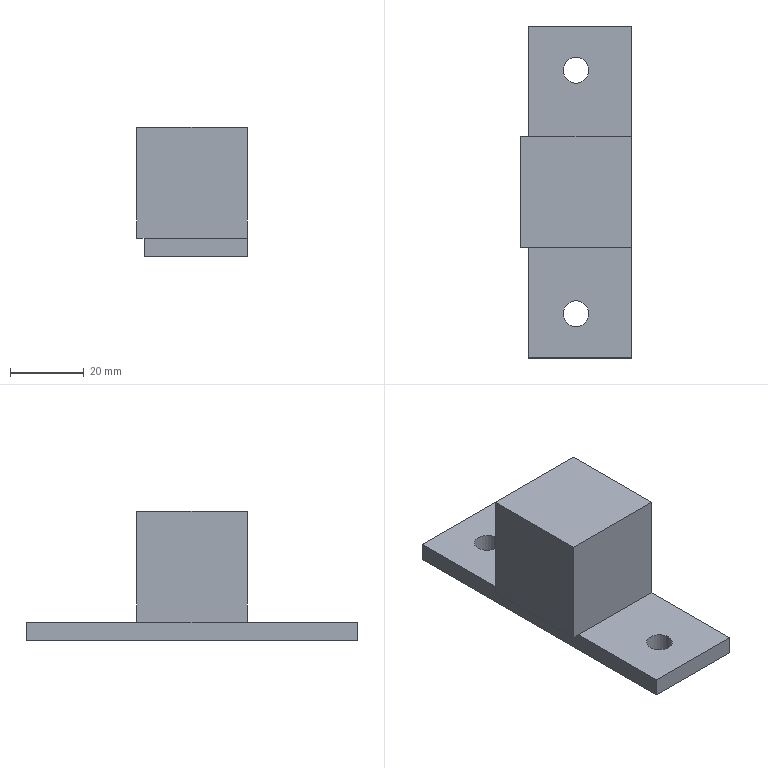Part | STEP file | diancitie | 1 solid | 14 faces | box 30 x 90 x 35 mm | volume 39215 mm3 | plane 12 | cylinder 2 | commonest cylinder face diameters 7 x2
STEP:
#1=CARTESIAN_POINT('',(0.,0.,0.));
#2=DIRECTION('',(0.,0.,1.));
#3=DIRECTION('',(1.,0.,0.));
#4=AXIS2_PLACEMENT_3D('',#1,#2,#3);
#5=CARTESIAN_POINT('',(-14.,-45.,0.));
#6=VERTEX_POINT('',#5);
#7=CARTESIAN_POINT('',(14.,-45.,0.));
#8=VERTEX_POINT('',#7);
#9=CARTESIAN_POINT('',(0.,-45.,0.));
#10=DIRECTION('',(1.,0.,0.));
#11=VECTOR('',#10,1.);
#12=LINE('',#9,#11);
#13=CARTESIAN_POINT('',(0.,0.,0.));
#14=DIRECTION('',(0.,0.,1.));
#15=DIRECTION('',(1.,0.,0.));
#16=AXIS2_PLACEMENT_3D('',#13,#14,#15);
#17=PLANE('',#16);
#18=CARTESIAN_POINT('',(0.,-45.));
#19=DIRECTION('',(1.,0.));
#20=VECTOR('',#19,1.);
#21=LINE('',#18,#20);
#22=(GEOMETRIC_REPRESENTATION_CONTEXT(2)PARAMETRIC_REPRESENTATION_CONTEXT()REPRESENTATION_CONTEXT('',''));
#23=DEFINITIONAL_REPRESENTATION('',(#21),#22);
#24=PCURVE('',#17,#23);
#25=CARTESIAN_POINT('',(-14.,-45.,5.));
#26=DIRECTION('',(0.,1.,0.));
#27=DIRECTION('',(0.,0.,1.));
#28=AXIS2_PLACEMENT_3D('',#25,#26,#27);
#29=PLANE('',#28);
#30=CARTESIAN_POINT('',(-5.,14.));
#31=DIRECTION('',(0.,1.));
#32=VECTOR('',#31,1.);
#33=LINE('',#30,#32);
#34=(GEOMETRIC_REPRESENTATION_CONTEXT(2)PARAMETRIC_REPRESENTATION_CONTEXT()REPRESENTATION_CONTEXT('',''));
#35=DEFINITIONAL_REPRESENTATION('',(#33),#34);
#36=PCURVE('',#29,#35);
#37=SURFACE_CURVE('',#12,(#24,#36),.PCURVE_S1.);
#38=EDGE_CURVE('',#6,#8,#37,.T.);
#39=ORIENTED_EDGE('',*,*,#38,.F.);
#40=CARTESIAN_POINT('',(-14.,45.,0.));
#41=VERTEX_POINT('',#40);
#42=CARTESIAN_POINT('',(-14.,0.,0.));
#43=DIRECTION('',(0.,-1.,0.));
#44=VECTOR('',#43,1.);
#45=LINE('',#42,#44);
#46=CARTESIAN_POINT('',(-14.,0.));
#47=DIRECTION('',(0.,-1.));
#48=VECTOR('',#47,1.);
#49=LINE('',#46,#48);
#50=(GEOMETRIC_REPRESENTATION_CONTEXT(2)PARAMETRIC_REPRESENTATION_CONTEXT()REPRESENTATION_CONTEXT('',''));
#51=DEFINITIONAL_REPRESENTATION('',(#49),#50);
#52=PCURVE('',#17,#51);
#53=CARTESIAN_POINT('',(-14.,45.,5.));
#54=DIRECTION('',(1.,0.,0.));
#55=DIRECTION('',(0.,1.,0.));
#56=AXIS2_PLACEMENT_3D('',#53,#54,#55);
#57=PLANE('',#56);
#58=CARTESIAN_POINT('',(-45.,-5.));
#59=DIRECTION('',(-1.,0.));
#60=VECTOR('',#59,1.);
#61=LINE('',#58,#60);
#62=(GEOMETRIC_REPRESENTATION_CONTEXT(2)PARAMETRIC_REPRESENTATION_CONTEXT()REPRESENTATION_CONTEXT('',''));
#63=DEFINITIONAL_REPRESENTATION('',(#61),#62);
#64=PCURVE('',#57,#63);
#65=SURFACE_CURVE('',#45,(#52,#64),.PCURVE_S1.);
#66=EDGE_CURVE('',#41,#6,#65,.T.);
#67=ORIENTED_EDGE('',*,*,#66,.F.);
#68=CARTESIAN_POINT('',(14.,45.,0.));
#69=VERTEX_POINT('',#68);
#70=CARTESIAN_POINT('',(0.,45.,0.));
#71=DIRECTION('',(-1.,0.,0.));
#72=VECTOR('',#71,1.);
#73=LINE('',#70,#72);
#74=CARTESIAN_POINT('',(0.,45.));
#75=DIRECTION('',(-1.,0.));
#76=VECTOR('',#75,1.);
#77=LINE('',#74,#76);
#78=(GEOMETRIC_REPRESENTATION_CONTEXT(2)PARAMETRIC_REPRESENTATION_CONTEXT()REPRESENTATION_CONTEXT('',''));
#79=DEFINITIONAL_REPRESENTATION('',(#77),#78);
#80=PCURVE('',#17,#79);
#81=CARTESIAN_POINT('',(-14.,45.,5.));
#82=DIRECTION('',(0.,-1.,0.));
#83=DIRECTION('',(0.,0.,-1.));
#84=AXIS2_PLACEMENT_3D('',#81,#82,#83);
#85=PLANE('',#84);
#86=CARTESIAN_POINT('',(5.,14.));
#87=DIRECTION('',(0.,-1.));
#88=VECTOR('',#87,1.);
#89=LINE('',#86,#88);
#90=(GEOMETRIC_REPRESENTATION_CONTEXT(2)PARAMETRIC_REPRESENTATION_CONTEXT()REPRESENTATION_CONTEXT('',''));
#91=DEFINITIONAL_REPRESENTATION('',(#89),#90);
#92=PCURVE('',#85,#91);
#93=SURFACE_CURVE('',#73,(#80,#92),.PCURVE_S1.);
#94=EDGE_CURVE('',#69,#41,#93,.T.);
#95=ORIENTED_EDGE('',*,*,#94,.F.);
#96=CARTESIAN_POINT('',(14.,0.,0.));
#97=DIRECTION('',(0.,1.,0.));
#98=VECTOR('',#97,1.);
#99=LINE('',#96,#98);
#100=CARTESIAN_POINT('',(14.,0.));
#101=DIRECTION('',(0.,1.));
#102=VECTOR('',#101,1.);
#103=LINE('',#100,#102);
#104=(GEOMETRIC_REPRESENTATION_CONTEXT(2)PARAMETRIC_REPRESENTATION_CONTEXT()REPRESENTATION_CONTEXT('',''));
#105=DEFINITIONAL_REPRESENTATION('',(#103),#104);
#106=PCURVE('',#17,#105);
#107=CARTESIAN_POINT('',(14.,45.,5.));
#108=DIRECTION('',(-1.,0.,0.));
#109=DIRECTION('',(0.,-1.,0.));
#110=AXIS2_PLACEMENT_3D('',#107,#108,#109);
#111=PLANE('',#110);
#112=CARTESIAN_POINT('',(45.,-5.));
#113=DIRECTION('',(-1.,0.));
#114=VECTOR('',#113,1.);
#115=LINE('',#112,#114);
#116=(GEOMETRIC_REPRESENTATION_CONTEXT(2)PARAMETRIC_REPRESENTATION_CONTEXT()REPRESENTATION_CONTEXT('',''));
#117=DEFINITIONAL_REPRESENTATION('',(#115),#116);
#118=PCURVE('',#111,#117);
#119=SURFACE_CURVE('',#99,(#106,#118),.PCURVE_S1.);
#120=EDGE_CURVE('',#8,#69,#119,.T.);
#121=ORIENTED_EDGE('',*,*,#120,.F.);
#122=EDGE_LOOP('',(#39,#67,#95,#121));
#123=FACE_BOUND('',#122,.T.);
#124=CARTESIAN_POINT('',(2.5,33.,0.));
#125=VERTEX_POINT('',#124);
#126=CARTESIAN_POINT('',(-1.,33.,0.));
#127=DIRECTION('',(0.,0.,-1.));
#128=DIRECTION('',(1.,0.,0.));
#129=AXIS2_PLACEMENT_3D('',#126,#127,#128);
#130=CIRCLE('',#129,3.5);
#131=CARTESIAN_POINT('',(2.5,33.));
#132=CARTESIAN_POINT('',(2.5,26.938));
#133=CARTESIAN_POINT('',(-2.75,29.969));
#134=CARTESIAN_POINT('',(-8.,33.));
#135=CARTESIAN_POINT('',(-2.75,36.031));
#136=CARTESIAN_POINT('',(2.5,39.062));
#137=CARTESIAN_POINT('',(2.5,33.));
#138=(BOUNDED_CURVE()B_SPLINE_CURVE(2,(#131,#132,#133,#134,#135,#136,#137),.UNSPECIFIED.,.T.,.F.)B_SPLINE_CURVE_WITH_KNOTS((1,2,2,2,2,1),(-2.094,0.,2.094,4.189,6.283,8.378),.UNSPECIFIED.)CURVE()GEOMETRIC_REPRESENTATION_ITEM()RATIONAL_B_SPLINE_CURVE((1.,0.5,1.,0.5,1.,0.5,1.))REPRESENTATION_ITEM(''));
#139=(GEOMETRIC_REPRESENTATION_CONTEXT(2)PARAMETRIC_REPRESENTATION_CONTEXT()REPRESENTATION_CONTEXT('',''));
#140=DEFINITIONAL_REPRESENTATION('',(#138),#139);
#141=PCURVE('',#17,#140);
#142=CARTESIAN_POINT('',(-1.,33.,0.));
#143=DIRECTION('',(0.,0.,1.));
#144=DIRECTION('',(1.,0.,0.));
#145=AXIS2_PLACEMENT_3D('',#142,#143,#144);
#146=CYLINDRICAL_SURFACE('',#145,3.5);
#147=CARTESIAN_POINT('',(6.283,0.));
#148=DIRECTION('',(-1.,0.));
#149=VECTOR('',#148,1.);
#150=LINE('',#147,#149);
#151=(GEOMETRIC_REPRESENTATION_CONTEXT(2)PARAMETRIC_REPRESENTATION_CONTEXT()REPRESENTATION_CONTEXT('',''));
#152=DEFINITIONAL_REPRESENTATION('',(#150),#151);
#153=PCURVE('',#146,#152);
#154=SURFACE_CURVE('',#130,(#141,#153),.PCURVE_S1.);
#155=EDGE_CURVE('',#125,#125,#154,.T.);
#156=ORIENTED_EDGE('',*,*,#155,.F.);
#157=EDGE_LOOP('',(#156));
#158=FACE_BOUND('',#157,.T.);
#159=CARTESIAN_POINT('',(2.5,-33.,0.));
#160=VERTEX_POINT('',#159);
#161=CARTESIAN_POINT('',(-1.,-33.,0.));
#162=DIRECTION('',(0.,0.,-1.));
#163=DIRECTION('',(1.,0.,0.));
#164=AXIS2_PLACEMENT_3D('',#161,#162,#163);
#165=CIRCLE('',#164,3.5);
#166=CARTESIAN_POINT('',(2.5,-33.));
#167=CARTESIAN_POINT('',(2.5,-39.062));
#168=CARTESIAN_POINT('',(-2.75,-36.031));
#169=CARTESIAN_POINT('',(-8.,-33.));
#170=CARTESIAN_POINT('',(-2.75,-29.969));
#171=CARTESIAN_POINT('',(2.5,-26.938));
#172=CARTESIAN_POINT('',(2.5,-33.));
#173=(BOUNDED_CURVE()B_SPLINE_CURVE(2,(#166,#167,#168,#169,#170,#171,#172),.UNSPECIFIED.,.T.,.F.)B_SPLINE_CURVE_WITH_KNOTS((1,2,2,2,2,1),(-2.094,0.,2.094,4.189,6.283,8.378),.UNSPECIFIED.)CURVE()GEOMETRIC_REPRESENTATION_ITEM()RATIONAL_B_SPLINE_CURVE((1.,0.5,1.,0.5,1.,0.5,1.))REPRESENTATION_ITEM(''));
#174=(GEOMETRIC_REPRESENTATION_CONTEXT(2)PARAMETRIC_REPRESENTATION_CONTEXT()REPRESENTATION_CONTEXT('',''));
#175=DEFINITIONAL_REPRESENTATION('',(#173),#174);
#176=PCURVE('',#17,#175);
#177=CARTESIAN_POINT('',(-1.,-33.,0.));
#178=DIRECTION('',(0.,0.,1.));
#179=DIRECTION('',(1.,0.,0.));
#180=AXIS2_PLACEMENT_3D('',#177,#178,#179);
#181=CYLINDRICAL_SURFACE('',#180,3.5);
#182=CARTESIAN_POINT('',(6.283,0.));
#183=DIRECTION('',(-1.,0.));
#184=VECTOR('',#183,1.);
#185=LINE('',#182,#184);
#186=(GEOMETRIC_REPRESENTATION_CONTEXT(2)PARAMETRIC_REPRESENTATION_CONTEXT()REPRESENTATION_CONTEXT('',''));
#187=DEFINITIONAL_REPRESENTATION('',(#185),#186);
#188=PCURVE('',#181,#187);
#189=SURFACE_CURVE('',#165,(#176,#188),.PCURVE_S1.);
#190=EDGE_CURVE('',#160,#160,#189,.T.);
#191=ORIENTED_EDGE('',*,*,#190,.F.);
#192=EDGE_LOOP('',(#191));
#193=FACE_BOUND('',#192,.T.);
#194=ADVANCED_FACE('',(#123,#158,#193),#17,.F.);
#195=CARTESIAN_POINT('',(14.,45.,5.));
#196=VERTEX_POINT('',#195);
#197=CARTESIAN_POINT('',(14.,45.,5.));
#198=DIRECTION('',(0.,0.,-1.));
#199=VECTOR('',#198,1.);
#200=LINE('',#197,#199);
#201=CARTESIAN_POINT('',(0.,0.));
#202=DIRECTION('',(0.,-1.));
#203=VECTOR('',#202,1.);
#204=LINE('',#201,#203);
#205=(GEOMETRIC_REPRESENTATION_CONTEXT(2)PARAMETRIC_REPRESENTATION_CONTEXT()REPRESENTATION_CONTEXT('',''));
#206=DEFINITIONAL_REPRESENTATION('',(#204),#205);
#207=PCURVE('',#111,#206);
#208=CARTESIAN_POINT('',(0.,28.));
#209=DIRECTION('',(1.,0.));
#210=VECTOR('',#209,1.);
#211=LINE('',#208,#210);
#212=(GEOMETRIC_REPRESENTATION_CONTEXT(2)PARAMETRIC_REPRESENTATION_CONTEXT()REPRESENTATION_CONTEXT('',''));
#213=DEFINITIONAL_REPRESENTATION('',(#211),#212);
#214=PCURVE('',#85,#213);
#215=SURFACE_CURVE('',#200,(#207,#214),.PCURVE_S1.);
#216=EDGE_CURVE('',#196,#69,#215,.T.);
#217=ORIENTED_EDGE('',*,*,#216,.F.);
#218=CARTESIAN_POINT('',(14.,15.,5.));
#219=VERTEX_POINT('',#218);
#220=CARTESIAN_POINT('',(14.,45.,5.));
#221=DIRECTION('',(0.,1.,0.));
#222=VECTOR('',#221,1.);
#223=LINE('',#220,#222);
#224=CARTESIAN_POINT('',(0.,0.));
#225=DIRECTION('',(-1.,0.));
#226=VECTOR('',#225,1.);
#227=LINE('',#224,#226);
#228=(GEOMETRIC_REPRESENTATION_CONTEXT(2)PARAMETRIC_REPRESENTATION_CONTEXT()REPRESENTATION_CONTEXT('',''));
#229=DEFINITIONAL_REPRESENTATION('',(#227),#228);
#230=PCURVE('',#111,#229);
#231=CARTESIAN_POINT('',(0.,0.,5.));
#232=DIRECTION('',(0.,0.,1.));
#233=DIRECTION('',(1.,0.,0.));
#234=AXIS2_PLACEMENT_3D('',#231,#232,#233);
#235=PLANE('',#234);
#236=CARTESIAN_POINT('',(14.,45.));
#237=DIRECTION('',(0.,1.));
#238=VECTOR('',#237,1.);
#239=LINE('',#236,#238);
#240=(GEOMETRIC_REPRESENTATION_CONTEXT(2)PARAMETRIC_REPRESENTATION_CONTEXT()REPRESENTATION_CONTEXT('',''));
#241=DEFINITIONAL_REPRESENTATION('',(#239),#240);
#242=PCURVE('',#235,#241);
#243=SURFACE_CURVE('',#223,(#230,#242),.PCURVE_S1.);
#244=EDGE_CURVE('',#219,#196,#243,.T.);
#245=ORIENTED_EDGE('',*,*,#244,.F.);
#246=CARTESIAN_POINT('',(14.,15.,35.));
#247=VERTEX_POINT('',#246);
#248=CARTESIAN_POINT('',(14.,15.,5.));
#249=DIRECTION('',(0.,0.,-1.));
#250=VECTOR('',#249,1.);
#251=LINE('',#248,#250);
#252=CARTESIAN_POINT('',(30.,0.));
#253=DIRECTION('',(0.,-1.));
#254=VECTOR('',#253,1.);
#255=LINE('',#252,#254);
#256=(GEOMETRIC_REPRESENTATION_CONTEXT(2)PARAMETRIC_REPRESENTATION_CONTEXT()REPRESENTATION_CONTEXT('',''));
#257=DEFINITIONAL_REPRESENTATION('',(#255),#256);
#258=PCURVE('',#111,#257);
#259=CARTESIAN_POINT('',(-16.,15.,35.));
#260=DIRECTION('',(0.,-1.,0.));
#261=DIRECTION('',(1.,0.,0.));
#262=AXIS2_PLACEMENT_3D('',#259,#260,#261);
#263=PLANE('',#262);
#264=CARTESIAN_POINT('',(30.,-30.));
#265=DIRECTION('',(0.,-1.));
#266=VECTOR('',#265,1.);
#267=LINE('',#264,#266);
#268=(GEOMETRIC_REPRESENTATION_CONTEXT(2)PARAMETRIC_REPRESENTATION_CONTEXT()REPRESENTATION_CONTEXT('',''));
#269=DEFINITIONAL_REPRESENTATION('',(#267),#268);
#270=PCURVE('',#263,#269);
#271=SURFACE_CURVE('',#251,(#258,#270),.PCURVE_S1.);
#272=EDGE_CURVE('',#247,#219,#271,.T.);
#273=ORIENTED_EDGE('',*,*,#272,.F.);
#274=CARTESIAN_POINT('',(14.,-15.,35.));
#275=VERTEX_POINT('',#274);
#276=CARTESIAN_POINT('',(14.,45.,35.));
#277=DIRECTION('',(0.,1.,0.));
#278=VECTOR('',#277,1.);
#279=LINE('',#276,#278);
#280=CARTESIAN_POINT('',(0.,30.));
#281=DIRECTION('',(-1.,0.));
#282=VECTOR('',#281,1.);
#283=LINE('',#280,#282);
#284=(GEOMETRIC_REPRESENTATION_CONTEXT(2)PARAMETRIC_REPRESENTATION_CONTEXT()REPRESENTATION_CONTEXT('',''));
#285=DEFINITIONAL_REPRESENTATION('',(#283),#284);
#286=PCURVE('',#111,#285);
#287=CARTESIAN_POINT('',(0.,0.,35.));
#288=DIRECTION('',(0.,0.,1.));
#289=DIRECTION('',(1.,0.,0.));
#290=AXIS2_PLACEMENT_3D('',#287,#288,#289);
#291=PLANE('',#290);
#292=CARTESIAN_POINT('',(14.,45.));
#293=DIRECTION('',(0.,1.));
#294=VECTOR('',#293,1.);
#295=LINE('',#292,#294);
#296=(GEOMETRIC_REPRESENTATION_CONTEXT(2)PARAMETRIC_REPRESENTATION_CONTEXT()REPRESENTATION_CONTEXT('',''));
#297=DEFINITIONAL_REPRESENTATION('',(#295),#296);
#298=PCURVE('',#291,#297);
#299=SURFACE_CURVE('',#279,(#286,#298),.PCURVE_S1.);
#300=EDGE_CURVE('',#275,#247,#299,.T.);
#301=ORIENTED_EDGE('',*,*,#300,.F.);
#302=CARTESIAN_POINT('',(14.,-15.,5.));
#303=VERTEX_POINT('',#302);
#304=CARTESIAN_POINT('',(14.,-15.,5.));
#305=DIRECTION('',(0.,0.,1.));
#306=VECTOR('',#305,1.);
#307=LINE('',#304,#306);
#308=CARTESIAN_POINT('',(60.,0.));
#309=DIRECTION('',(0.,1.));
#310=VECTOR('',#309,1.);
#311=LINE('',#308,#310);
#312=(GEOMETRIC_REPRESENTATION_CONTEXT(2)PARAMETRIC_REPRESENTATION_CONTEXT()REPRESENTATION_CONTEXT('',''));
#313=DEFINITIONAL_REPRESENTATION('',(#311),#312);
#314=PCURVE('',#111,#313);
#315=CARTESIAN_POINT('',(-16.,-15.,35.));
#316=DIRECTION('',(0.,1.,0.));
#317=DIRECTION('',(0.,0.,1.));
#318=AXIS2_PLACEMENT_3D('',#315,#316,#317);
#319=PLANE('',#318);
#320=CARTESIAN_POINT('',(-30.,30.));
#321=DIRECTION('',(1.,0.));
#322=VECTOR('',#321,1.);
#323=LINE('',#320,#322);
#324=(GEOMETRIC_REPRESENTATION_CONTEXT(2)PARAMETRIC_REPRESENTATION_CONTEXT()REPRESENTATION_CONTEXT('',''));
#325=DEFINITIONAL_REPRESENTATION('',(#323),#324);
#326=PCURVE('',#319,#325);
#327=SURFACE_CURVE('',#307,(#314,#326),.PCURVE_S1.);
#328=EDGE_CURVE('',#303,#275,#327,.T.);
#329=ORIENTED_EDGE('',*,*,#328,.F.);
#330=CARTESIAN_POINT('',(14.,-45.,5.));
#331=VERTEX_POINT('',#330);
#332=CARTESIAN_POINT('',(14.,45.,5.));
#333=DIRECTION('',(0.,1.,0.));
#334=VECTOR('',#333,1.);
#335=LINE('',#332,#334);
#336=CARTESIAN_POINT('',(0.,0.));
#337=DIRECTION('',(-1.,0.));
#338=VECTOR('',#337,1.);
#339=LINE('',#336,#338);
#340=(GEOMETRIC_REPRESENTATION_CONTEXT(2)PARAMETRIC_REPRESENTATION_CONTEXT()REPRESENTATION_CONTEXT('',''));
#341=DEFINITIONAL_REPRESENTATION('',(#339),#340);
#342=PCURVE('',#111,#341);
#343=CARTESIAN_POINT('',(0.,0.,5.));
#344=DIRECTION('',(0.,0.,1.));
#345=DIRECTION('',(1.,0.,0.));
#346=AXIS2_PLACEMENT_3D('',#343,#344,#345);
#347=PLANE('',#346);
#348=CARTESIAN_POINT('',(14.,45.));
#349=DIRECTION('',(0.,1.));
#350=VECTOR('',#349,1.);
#351=LINE('',#348,#350);
#352=(GEOMETRIC_REPRESENTATION_CONTEXT(2)PARAMETRIC_REPRESENTATION_CONTEXT()REPRESENTATION_CONTEXT('',''));
#353=DEFINITIONAL_REPRESENTATION('',(#351),#352);
#354=PCURVE('',#347,#353);
#355=SURFACE_CURVE('',#335,(#342,#354),.PCURVE_S1.);
#356=EDGE_CURVE('',#331,#303,#355,.T.);
#357=ORIENTED_EDGE('',*,*,#356,.F.);
#358=CARTESIAN_POINT('',(14.,-45.,5.));
#359=DIRECTION('',(0.,0.,1.));
#360=VECTOR('',#359,1.);
#361=LINE('',#358,#360);
#362=CARTESIAN_POINT('',(90.,0.));
#363=DIRECTION('',(0.,1.));
#364=VECTOR('',#363,1.);
#365=LINE('',#362,#364);
#366=(GEOMETRIC_REPRESENTATION_CONTEXT(2)PARAMETRIC_REPRESENTATION_CONTEXT()REPRESENTATION_CONTEXT('',''));
#367=DEFINITIONAL_REPRESENTATION('',(#365),#366);
#368=PCURVE('',#111,#367);
#369=CARTESIAN_POINT('',(0.,28.));
#370=DIRECTION('',(1.,0.));
#371=VECTOR('',#370,1.);
#372=LINE('',#369,#371);
#373=(GEOMETRIC_REPRESENTATION_CONTEXT(2)PARAMETRIC_REPRESENTATION_CONTEXT()REPRESENTATION_CONTEXT('',''));
#374=DEFINITIONAL_REPRESENTATION('',(#372),#373);
#375=PCURVE('',#29,#374);
#376=SURFACE_CURVE('',#361,(#368,#375),.PCURVE_S1.);
#377=EDGE_CURVE('',#8,#331,#376,.T.);
#378=ORIENTED_EDGE('',*,*,#377,.F.);
#379=ORIENTED_EDGE('',*,*,#120,.T.);
#380=EDGE_LOOP('',(#217,#245,#273,#301,#329,#357,#378,#379));
#381=FACE_BOUND('',#380,.T.);
#382=ADVANCED_FACE('',(#381),#111,.F.);
#383=ORIENTED_EDGE('',*,*,#377,.T.);
#384=CARTESIAN_POINT('',(-14.,-45.,5.));
#385=VERTEX_POINT('',#384);
#386=CARTESIAN_POINT('',(-14.,-45.,5.));
#387=DIRECTION('',(1.,0.,0.));
#388=VECTOR('',#387,1.);
#389=LINE('',#386,#388);
#390=CARTESIAN_POINT('',(0.,0.));
#391=DIRECTION('',(0.,1.));
#392=VECTOR('',#391,1.);
#393=LINE('',#390,#392);
#394=(GEOMETRIC_REPRESENTATION_CONTEXT(2)PARAMETRIC_REPRESENTATION_CONTEXT()REPRESENTATION_CONTEXT('',''));
#395=DEFINITIONAL_REPRESENTATION('',(#393),#394);
#396=PCURVE('',#29,#395);
#397=CARTESIAN_POINT('',(-14.,-45.));
#398=DIRECTION('',(1.,0.));
#399=VECTOR('',#398,1.);
#400=LINE('',#397,#399);
#401=(GEOMETRIC_REPRESENTATION_CONTEXT(2)PARAMETRIC_REPRESENTATION_CONTEXT()REPRESENTATION_CONTEXT('',''));
#402=DEFINITIONAL_REPRESENTATION('',(#400),#401);
#403=PCURVE('',#347,#402);
#404=SURFACE_CURVE('',#389,(#396,#403),.PCURVE_S1.);
#405=EDGE_CURVE('',#385,#331,#404,.T.);
#406=ORIENTED_EDGE('',*,*,#405,.F.);
#407=CARTESIAN_POINT('',(-14.,-45.,5.));
#408=DIRECTION('',(0.,0.,1.));
#409=VECTOR('',#408,1.);
#410=LINE('',#407,#409);
#411=CARTESIAN_POINT('',(0.,0.));
#412=DIRECTION('',(1.,0.));
#413=VECTOR('',#412,1.);
#414=LINE('',#411,#413);
#415=(GEOMETRIC_REPRESENTATION_CONTEXT(2)PARAMETRIC_REPRESENTATION_CONTEXT()REPRESENTATION_CONTEXT('',''));
#416=DEFINITIONAL_REPRESENTATION('',(#414),#415);
#417=PCURVE('',#29,#416);
#418=CARTESIAN_POINT('',(-90.,0.));
#419=DIRECTION('',(0.,1.));
#420=VECTOR('',#419,1.);
#421=LINE('',#418,#420);
#422=(GEOMETRIC_REPRESENTATION_CONTEXT(2)PARAMETRIC_REPRESENTATION_CONTEXT()REPRESENTATION_CONTEXT('',''));
#423=DEFINITIONAL_REPRESENTATION('',(#421),#422);
#424=PCURVE('',#57,#423);
#425=SURFACE_CURVE('',#410,(#417,#424),.PCURVE_S1.);
#426=EDGE_CURVE('',#6,#385,#425,.T.);
#427=ORIENTED_EDGE('',*,*,#426,.F.);
#428=ORIENTED_EDGE('',*,*,#38,.T.);
#429=EDGE_LOOP('',(#383,#406,#427,#428));
#430=FACE_BOUND('',#429,.T.);
#431=ADVANCED_FACE('',(#430),#29,.F.);
#432=ORIENTED_EDGE('',*,*,#426,.T.);
#433=CARTESIAN_POINT('',(-14.,-15.,5.));
#434=VERTEX_POINT('',#433);
#435=CARTESIAN_POINT('',(-14.,45.,5.));
#436=DIRECTION('',(0.,-1.,0.));
#437=VECTOR('',#436,1.);
#438=LINE('',#435,#437);
#439=CARTESIAN_POINT('',(0.,0.));
#440=DIRECTION('',(-1.,0.));
#441=VECTOR('',#440,1.);
#442=LINE('',#439,#441);
#443=(GEOMETRIC_REPRESENTATION_CONTEXT(2)PARAMETRIC_REPRESENTATION_CONTEXT()REPRESENTATION_CONTEXT('',''));
#444=DEFINITIONAL_REPRESENTATION('',(#442),#443);
#445=PCURVE('',#57,#444);
#446=CARTESIAN_POINT('',(-14.,45.));
#447=DIRECTION('',(0.,-1.));
#448=VECTOR('',#447,1.);
#449=LINE('',#446,#448);
#450=(GEOMETRIC_REPRESENTATION_CONTEXT(2)PARAMETRIC_REPRESENTATION_CONTEXT()REPRESENTATION_CONTEXT('',''));
#451=DEFINITIONAL_REPRESENTATION('',(#449),#450);
#452=PCURVE('',#347,#451);
#453=SURFACE_CURVE('',#438,(#445,#452),.PCURVE_S1.);
#454=EDGE_CURVE('',#434,#385,#453,.T.);
#455=ORIENTED_EDGE('',*,*,#454,.F.);
#456=CARTESIAN_POINT('',(-14.,15.,5.));
#457=VERTEX_POINT('',#456);
#458=CARTESIAN_POINT('',(-14.,45.,5.));
#459=DIRECTION('',(0.,-1.,0.));
#460=VECTOR('',#459,1.);
#461=LINE('',#458,#460);
#462=CARTESIAN_POINT('',(0.,0.));
#463=DIRECTION('',(-1.,0.));
#464=VECTOR('',#463,1.);
#465=LINE('',#462,#464);
#466=(GEOMETRIC_REPRESENTATION_CONTEXT(2)PARAMETRIC_REPRESENTATION_CONTEXT()REPRESENTATION_CONTEXT('',''));
#467=DEFINITIONAL_REPRESENTATION('',(#465),#466);
#468=PCURVE('',#57,#467);
#469=CARTESIAN_POINT('',(0.,0.,5.));
#470=DIRECTION('',(0.,0.,1.));
#471=DIRECTION('',(1.,0.,0.));
#472=AXIS2_PLACEMENT_3D('',#469,#470,#471);
#473=PLANE('',#472);
#474=CARTESIAN_POINT('',(-14.,45.));
#475=DIRECTION('',(0.,-1.));
#476=VECTOR('',#475,1.);
#477=LINE('',#474,#476);
#478=(GEOMETRIC_REPRESENTATION_CONTEXT(2)PARAMETRIC_REPRESENTATION_CONTEXT()REPRESENTATION_CONTEXT('',''));
#479=DEFINITIONAL_REPRESENTATION('',(#477),#478);
#480=PCURVE('',#473,#479);
#481=SURFACE_CURVE('',#461,(#468,#480),.PCURVE_S1.);
#482=EDGE_CURVE('',#457,#434,#481,.T.);
#483=ORIENTED_EDGE('',*,*,#482,.F.);
#484=CARTESIAN_POINT('',(-14.,45.,5.));
#485=VERTEX_POINT('',#484);
#486=CARTESIAN_POINT('',(-14.,45.,5.));
#487=DIRECTION('',(0.,-1.,0.));
#488=VECTOR('',#487,1.);
#489=LINE('',#486,#488);
#490=CARTESIAN_POINT('',(0.,0.));
#491=DIRECTION('',(-1.,0.));
#492=VECTOR('',#491,1.);
#493=LINE('',#490,#492);
#494=(GEOMETRIC_REPRESENTATION_CONTEXT(2)PARAMETRIC_REPRESENTATION_CONTEXT()REPRESENTATION_CONTEXT('',''));
#495=DEFINITIONAL_REPRESENTATION('',(#493),#494);
#496=PCURVE('',#57,#495);
#497=CARTESIAN_POINT('',(-14.,45.));
#498=DIRECTION('',(0.,-1.));
#499=VECTOR('',#498,1.);
#500=LINE('',#497,#499);
#501=(GEOMETRIC_REPRESENTATION_CONTEXT(2)PARAMETRIC_REPRESENTATION_CONTEXT()REPRESENTATION_CONTEXT('',''));
#502=DEFINITIONAL_REPRESENTATION('',(#500),#501);
#503=PCURVE('',#235,#502);
#504=SURFACE_CURVE('',#489,(#496,#503),.PCURVE_S1.);
#505=EDGE_CURVE('',#485,#457,#504,.T.);
#506=ORIENTED_EDGE('',*,*,#505,.F.);
#507=CARTESIAN_POINT('',(-14.,45.,5.));
#508=DIRECTION('',(0.,0.,1.));
#509=VECTOR('',#508,1.);
#510=LINE('',#507,#509);
#511=CARTESIAN_POINT('',(0.,0.));
#512=DIRECTION('',(0.,1.));
#513=VECTOR('',#512,1.);
#514=LINE('',#511,#513);
#515=(GEOMETRIC_REPRESENTATION_CONTEXT(2)PARAMETRIC_REPRESENTATION_CONTEXT()REPRESENTATION_CONTEXT('',''));
#516=DEFINITIONAL_REPRESENTATION('',(#514),#515);
#517=PCURVE('',#57,#516);
#518=CARTESIAN_POINT('',(0.,0.));
#519=DIRECTION('',(-1.,0.));
#520=VECTOR('',#519,1.);
#521=LINE('',#518,#520);
#522=(GEOMETRIC_REPRESENTATION_CONTEXT(2)PARAMETRIC_REPRESENTATION_CONTEXT()REPRESENTATION_CONTEXT('',''));
#523=DEFINITIONAL_REPRESENTATION('',(#521),#522);
#524=PCURVE('',#85,#523);
#525=SURFACE_CURVE('',#510,(#517,#524),.PCURVE_S1.);
#526=EDGE_CURVE('',#41,#485,#525,.T.);
#527=ORIENTED_EDGE('',*,*,#526,.F.);
#528=ORIENTED_EDGE('',*,*,#66,.T.);
#529=EDGE_LOOP('',(#432,#455,#483,#506,#527,#528));
#530=FACE_BOUND('',#529,.T.);
#531=ADVANCED_FACE('',(#530),#57,.F.);
#532=ORIENTED_EDGE('',*,*,#526,.T.);
#533=CARTESIAN_POINT('',(-14.,45.,5.));
#534=DIRECTION('',(-1.,0.,0.));
#535=VECTOR('',#534,1.);
#536=LINE('',#533,#535);
#537=CARTESIAN_POINT('',(0.,0.));
#538=DIRECTION('',(0.,-1.));
#539=VECTOR('',#538,1.);
#540=LINE('',#537,#539);
#541=(GEOMETRIC_REPRESENTATION_CONTEXT(2)PARAMETRIC_REPRESENTATION_CONTEXT()REPRESENTATION_CONTEXT('',''));
#542=DEFINITIONAL_REPRESENTATION('',(#540),#541);
#543=PCURVE('',#85,#542);
#544=CARTESIAN_POINT('',(-14.,45.));
#545=DIRECTION('',(-1.,0.));
#546=VECTOR('',#545,1.);
#547=LINE('',#544,#546);
#548=(GEOMETRIC_REPRESENTATION_CONTEXT(2)PARAMETRIC_REPRESENTATION_CONTEXT()REPRESENTATION_CONTEXT('',''));
#549=DEFINITIONAL_REPRESENTATION('',(#547),#548);
#550=PCURVE('',#235,#549);
#551=SURFACE_CURVE('',#536,(#543,#550),.PCURVE_S1.);
#552=EDGE_CURVE('',#196,#485,#551,.T.);
#553=ORIENTED_EDGE('',*,*,#552,.F.);
#554=ORIENTED_EDGE('',*,*,#216,.T.);
#555=ORIENTED_EDGE('',*,*,#94,.T.);
#556=EDGE_LOOP('',(#532,#553,#554,#555));
#557=FACE_BOUND('',#556,.T.);
#558=ADVANCED_FACE('',(#557),#85,.F.);
#559=ORIENTED_EDGE('',*,*,#155,.F.);
#560=CARTESIAN_POINT('',(2.5,33.,5.));
#561=VERTEX_POINT('',#560);
#562=CARTESIAN_POINT('',(2.5,33.,0.));
#563=CARTESIAN_POINT('',(2.5,33.,5.));
#564=B_SPLINE_CURVE_WITH_KNOTS('',1,(#562,#563),.UNSPECIFIED.,.F.,.F.,(2,2),(0.,5.),.PIECEWISE_BEZIER_KNOTS.);
#565=CARTESIAN_POINT('',(6.283,0.));
#566=DIRECTION('',(0.,1.));
#567=VECTOR('',#566,1.);
#568=LINE('',#565,#567);
#569=(GEOMETRIC_REPRESENTATION_CONTEXT(2)PARAMETRIC_REPRESENTATION_CONTEXT()REPRESENTATION_CONTEXT('',''));
#570=DEFINITIONAL_REPRESENTATION('',(#568),#569);
#571=PCURVE('',#146,#570);
#572=CARTESIAN_POINT('',(0.,0.));
#573=DIRECTION('',(0.,1.));
#574=VECTOR('',#573,1.);
#575=LINE('',#572,#574);
#576=(GEOMETRIC_REPRESENTATION_CONTEXT(2)PARAMETRIC_REPRESENTATION_CONTEXT()REPRESENTATION_CONTEXT('',''));
#577=DEFINITIONAL_REPRESENTATION('',(#575),#576);
#578=PCURVE('',#146,#577);
#579=SEAM_CURVE('',#564,(#571,#578),.PCURVE_S1.);
#580=EDGE_CURVE('',#125,#561,#579,.T.);
#581=ORIENTED_EDGE('',*,*,#580,.T.);
#582=CARTESIAN_POINT('',(-1.,33.,5.));
#583=DIRECTION('',(0.,0.,-1.));
#584=DIRECTION('',(1.,0.,0.));
#585=AXIS2_PLACEMENT_3D('',#582,#583,#584);
#586=CIRCLE('',#585,3.5);
#587=CARTESIAN_POINT('',(6.283,5.));
#588=DIRECTION('',(-1.,0.));
#589=VECTOR('',#588,1.);
#590=LINE('',#587,#589);
#591=(GEOMETRIC_REPRESENTATION_CONTEXT(2)PARAMETRIC_REPRESENTATION_CONTEXT()REPRESENTATION_CONTEXT('',''));
#592=DEFINITIONAL_REPRESENTATION('',(#590),#591);
#593=PCURVE('',#146,#592);
#594=CARTESIAN_POINT('',(2.5,33.));
#595=CARTESIAN_POINT('',(2.5,26.938));
#596=CARTESIAN_POINT('',(-2.75,29.969));
#597=CARTESIAN_POINT('',(-8.,33.));
#598=CARTESIAN_POINT('',(-2.75,36.031));
#599=CARTESIAN_POINT('',(2.5,39.062));
#600=CARTESIAN_POINT('',(2.5,33.));
#601=(BOUNDED_CURVE()B_SPLINE_CURVE(2,(#594,#595,#596,#597,#598,#599,#600),.UNSPECIFIED.,.T.,.F.)B_SPLINE_CURVE_WITH_KNOTS((1,2,2,2,2,1),(-2.094,0.,2.094,4.189,6.283,8.378),.UNSPECIFIED.)CURVE()GEOMETRIC_REPRESENTATION_ITEM()RATIONAL_B_SPLINE_CURVE((1.,0.5,1.,0.5,1.,0.5,1.))REPRESENTATION_ITEM(''));
#602=(GEOMETRIC_REPRESENTATION_CONTEXT(2)PARAMETRIC_REPRESENTATION_CONTEXT()REPRESENTATION_CONTEXT('',''));
#603=DEFINITIONAL_REPRESENTATION('',(#601),#602);
#604=PCURVE('',#235,#603);
#605=SURFACE_CURVE('',#586,(#593,#604),.PCURVE_S1.);
#606=EDGE_CURVE('',#561,#561,#605,.T.);
#607=ORIENTED_EDGE('',*,*,#606,.T.);
#608=ORIENTED_EDGE('',*,*,#580,.F.);
#609=EDGE_LOOP('',(#559,#581,#607,#608));
#610=FACE_BOUND('',#609,.F.);
#611=ADVANCED_FACE('',(#610),#146,.F.);
#612=ORIENTED_EDGE('',*,*,#190,.F.);
#613=CARTESIAN_POINT('',(2.5,-33.,5.));
#614=VERTEX_POINT('',#613);
#615=CARTESIAN_POINT('',(2.5,-33.,0.));
#616=CARTESIAN_POINT('',(2.5,-33.,5.));
#617=B_SPLINE_CURVE_WITH_KNOTS('',1,(#615,#616),.UNSPECIFIED.,.F.,.F.,(2,2),(0.,5.),.PIECEWISE_BEZIER_KNOTS.);
#618=CARTESIAN_POINT('',(6.283,0.));
#619=DIRECTION('',(0.,1.));
#620=VECTOR('',#619,1.);
#621=LINE('',#618,#620);
#622=(GEOMETRIC_REPRESENTATION_CONTEXT(2)PARAMETRIC_REPRESENTATION_CONTEXT()REPRESENTATION_CONTEXT('',''));
#623=DEFINITIONAL_REPRESENTATION('',(#621),#622);
#624=PCURVE('',#181,#623);
#625=CARTESIAN_POINT('',(0.,0.));
#626=DIRECTION('',(0.,1.));
#627=VECTOR('',#626,1.);
#628=LINE('',#625,#627);
#629=(GEOMETRIC_REPRESENTATION_CONTEXT(2)PARAMETRIC_REPRESENTATION_CONTEXT()REPRESENTATION_CONTEXT('',''));
#630=DEFINITIONAL_REPRESENTATION('',(#628),#629);
#631=PCURVE('',#181,#630);
#632=SEAM_CURVE('',#617,(#624,#631),.PCURVE_S1.);
#633=EDGE_CURVE('',#160,#614,#632,.T.);
#634=ORIENTED_EDGE('',*,*,#633,.T.);
#635=CARTESIAN_POINT('',(-1.,-33.,5.));
#636=DIRECTION('',(0.,0.,-1.));
#637=DIRECTION('',(1.,0.,0.));
#638=AXIS2_PLACEMENT_3D('',#635,#636,#637);
#639=CIRCLE('',#638,3.5);
#640=CARTESIAN_POINT('',(6.283,5.));
#641=DIRECTION('',(-1.,0.));
#642=VECTOR('',#641,1.);
#643=LINE('',#640,#642);
#644=(GEOMETRIC_REPRESENTATION_CONTEXT(2)PARAMETRIC_REPRESENTATION_CONTEXT()REPRESENTATION_CONTEXT('',''));
#645=DEFINITIONAL_REPRESENTATION('',(#643),#644);
#646=PCURVE('',#181,#645);
#647=CARTESIAN_POINT('',(2.5,-33.));
#648=CARTESIAN_POINT('',(2.5,-39.062));
#649=CARTESIAN_POINT('',(-2.75,-36.031));
#650=CARTESIAN_POINT('',(-8.,-33.));
#651=CARTESIAN_POINT('',(-2.75,-29.969));
#652=CARTESIAN_POINT('',(2.5,-26.938));
#653=CARTESIAN_POINT('',(2.5,-33.));
#654=(BOUNDED_CURVE()B_SPLINE_CURVE(2,(#647,#648,#649,#650,#651,#652,#653),.UNSPECIFIED.,.T.,.F.)B_SPLINE_CURVE_WITH_KNOTS((1,2,2,2,2,1),(-2.094,0.,2.094,4.189,6.283,8.378),.UNSPECIFIED.)CURVE()GEOMETRIC_REPRESENTATION_ITEM()RATIONAL_B_SPLINE_CURVE((1.,0.5,1.,0.5,1.,0.5,1.))REPRESENTATION_ITEM(''));
#655=(GEOMETRIC_REPRESENTATION_CONTEXT(2)PARAMETRIC_REPRESENTATION_CONTEXT()REPRESENTATION_CONTEXT('',''));
#656=DEFINITIONAL_REPRESENTATION('',(#654),#655);
#657=PCURVE('',#347,#656);
#658=SURFACE_CURVE('',#639,(#646,#657),.PCURVE_S1.);
#659=EDGE_CURVE('',#614,#614,#658,.T.);
#660=ORIENTED_EDGE('',*,*,#659,.T.);
#661=ORIENTED_EDGE('',*,*,#633,.F.);
#662=EDGE_LOOP('',(#612,#634,#660,#661));
#663=FACE_BOUND('',#662,.F.);
#664=ADVANCED_FACE('',(#663),#181,.F.);
#665=ORIENTED_EDGE('',*,*,#606,.T.);
#666=EDGE_LOOP('',(#665));
#667=FACE_BOUND('',#666,.T.);
#668=ORIENTED_EDGE('',*,*,#552,.T.);
#669=ORIENTED_EDGE('',*,*,#505,.T.);
#670=CARTESIAN_POINT('',(0.,15.,5.));
#671=DIRECTION('',(1.,0.,0.));
#672=VECTOR('',#671,1.);
#673=LINE('',#670,#672);
#674=CARTESIAN_POINT('',(0.,15.));
#675=DIRECTION('',(1.,0.));
#676=VECTOR('',#675,1.);
#677=LINE('',#674,#676);
#678=(GEOMETRIC_REPRESENTATION_CONTEXT(2)PARAMETRIC_REPRESENTATION_CONTEXT()REPRESENTATION_CONTEXT('',''));
#679=DEFINITIONAL_REPRESENTATION('',(#677),#678);
#680=PCURVE('',#235,#679);
#681=CARTESIAN_POINT('',(16.,-30.));
#682=DIRECTION('',(1.,0.));
#683=VECTOR('',#682,1.);
#684=LINE('',#681,#683);
#685=(GEOMETRIC_REPRESENTATION_CONTEXT(2)PARAMETRIC_REPRESENTATION_CONTEXT()REPRESENTATION_CONTEXT('',''));
#686=DEFINITIONAL_REPRESENTATION('',(#684),#685);
#687=PCURVE('',#263,#686);
#688=SURFACE_CURVE('',#673,(#680,#687),.PCURVE_S1.);
#689=EDGE_CURVE('',#457,#219,#688,.T.);
#690=ORIENTED_EDGE('',*,*,#689,.T.);
#691=ORIENTED_EDGE('',*,*,#244,.T.);
#692=EDGE_LOOP('',(#668,#669,#690,#691));
#693=FACE_BOUND('',#692,.T.);
#694=ADVANCED_FACE('',(#667,#693),#235,.T.);
#695=CARTESIAN_POINT('',(-16.,15.,5.));
#696=VERTEX_POINT('',#695);
#697=CARTESIAN_POINT('',(-16.,15.,5.));
#698=DIRECTION('',(1.,0.,0.));
#699=VECTOR('',#698,1.);
#700=LINE('',#697,#699);
#701=CARTESIAN_POINT('',(0.,-30.));
#702=DIRECTION('',(1.,0.));
#703=VECTOR('',#702,1.);
#704=LINE('',#701,#703);
#705=(GEOMETRIC_REPRESENTATION_CONTEXT(2)PARAMETRIC_REPRESENTATION_CONTEXT()REPRESENTATION_CONTEXT('',''));
#706=DEFINITIONAL_REPRESENTATION('',(#704),#705);
#707=PCURVE('',#263,#706);
#708=CARTESIAN_POINT('',(-16.,15.));
#709=DIRECTION('',(1.,0.));
#710=VECTOR('',#709,1.);
#711=LINE('',#708,#710);
#712=(GEOMETRIC_REPRESENTATION_CONTEXT(2)PARAMETRIC_REPRESENTATION_CONTEXT()REPRESENTATION_CONTEXT('',''));
#713=DEFINITIONAL_REPRESENTATION('',(#711),#712);
#714=PCURVE('',#473,#713);
#715=SURFACE_CURVE('',#700,(#707,#714),.PCURVE_S1.);
#716=EDGE_CURVE('',#696,#457,#715,.T.);
#717=ORIENTED_EDGE('',*,*,#716,.F.);
#718=CARTESIAN_POINT('',(-16.,15.,35.));
#719=VERTEX_POINT('',#718);
#720=CARTESIAN_POINT('',(-16.,15.,35.));
#721=DIRECTION('',(0.,0.,-1.));
#722=VECTOR('',#721,1.);
#723=LINE('',#720,#722);
#724=CARTESIAN_POINT('',(0.,0.));
#725=DIRECTION('',(0.,-1.));
#726=VECTOR('',#725,1.);
#727=LINE('',#724,#726);
#728=(GEOMETRIC_REPRESENTATION_CONTEXT(2)PARAMETRIC_REPRESENTATION_CONTEXT()REPRESENTATION_CONTEXT('',''));
#729=DEFINITIONAL_REPRESENTATION('',(#727),#728);
#730=PCURVE('',#263,#729);
#731=CARTESIAN_POINT('',(-16.,15.,35.));
#732=DIRECTION('',(1.,0.,0.));
#733=DIRECTION('',(0.,1.,0.));
#734=AXIS2_PLACEMENT_3D('',#731,#732,#733);
#735=PLANE('',#734);
#736=CARTESIAN_POINT('',(0.,0.));
#737=DIRECTION('',(0.,-1.));
#738=VECTOR('',#737,1.);
#739=LINE('',#736,#738);
#740=(GEOMETRIC_REPRESENTATION_CONTEXT(2)PARAMETRIC_REPRESENTATION_CONTEXT()REPRESENTATION_CONTEXT('',''));
#741=DEFINITIONAL_REPRESENTATION('',(#739),#740);
#742=PCURVE('',#735,#741);
#743=SURFACE_CURVE('',#723,(#730,#742),.PCURVE_S1.);
#744=EDGE_CURVE('',#719,#696,#743,.T.);
#745=ORIENTED_EDGE('',*,*,#744,.F.);
#746=CARTESIAN_POINT('',(-16.,15.,35.));
#747=DIRECTION('',(-1.,0.,0.));
#748=VECTOR('',#747,1.);
#749=LINE('',#746,#748);
#750=CARTESIAN_POINT('',(0.,0.));
#751=DIRECTION('',(-1.,0.));
#752=VECTOR('',#751,1.);
#753=LINE('',#750,#752);
#754=(GEOMETRIC_REPRESENTATION_CONTEXT(2)PARAMETRIC_REPRESENTATION_CONTEXT()REPRESENTATION_CONTEXT('',''));
#755=DEFINITIONAL_REPRESENTATION('',(#753),#754);
#756=PCURVE('',#263,#755);
#757=CARTESIAN_POINT('',(-16.,15.));
#758=DIRECTION('',(-1.,0.));
#759=VECTOR('',#758,1.);
#760=LINE('',#757,#759);
#761=(GEOMETRIC_REPRESENTATION_CONTEXT(2)PARAMETRIC_REPRESENTATION_CONTEXT()REPRESENTATION_CONTEXT('',''));
#762=DEFINITIONAL_REPRESENTATION('',(#760),#761);
#763=PCURVE('',#291,#762);
#764=SURFACE_CURVE('',#749,(#756,#763),.PCURVE_S1.);
#765=EDGE_CURVE('',#247,#719,#764,.T.);
#766=ORIENTED_EDGE('',*,*,#765,.F.);
#767=ORIENTED_EDGE('',*,*,#272,.T.);
#768=ORIENTED_EDGE('',*,*,#689,.F.);
#769=EDGE_LOOP('',(#717,#745,#766,#767,#768));
#770=FACE_BOUND('',#769,.T.);
#771=ADVANCED_FACE('',(#770),#263,.F.);
#772=ORIENTED_EDGE('',*,*,#300,.T.);
#773=ORIENTED_EDGE('',*,*,#765,.T.);
#774=CARTESIAN_POINT('',(-16.,-15.,35.));
#775=VERTEX_POINT('',#774);
#776=CARTESIAN_POINT('',(-16.,0.,35.));
#777=DIRECTION('',(0.,-1.,0.));
#778=VECTOR('',#777,1.);
#779=LINE('',#776,#778);
#780=CARTESIAN_POINT('',(-16.,0.));
#781=DIRECTION('',(0.,-1.));
#782=VECTOR('',#781,1.);
#783=LINE('',#780,#782);
#784=(GEOMETRIC_REPRESENTATION_CONTEXT(2)PARAMETRIC_REPRESENTATION_CONTEXT()REPRESENTATION_CONTEXT('',''));
#785=DEFINITIONAL_REPRESENTATION('',(#783),#784);
#786=PCURVE('',#291,#785);
#787=CARTESIAN_POINT('',(-15.,0.));
#788=DIRECTION('',(-1.,0.));
#789=VECTOR('',#788,1.);
#790=LINE('',#787,#789);
#791=(GEOMETRIC_REPRESENTATION_CONTEXT(2)PARAMETRIC_REPRESENTATION_CONTEXT()REPRESENTATION_CONTEXT('',''));
#792=DEFINITIONAL_REPRESENTATION('',(#790),#791);
#793=PCURVE('',#735,#792);
#794=SURFACE_CURVE('',#779,(#786,#793),.PCURVE_S1.);
#795=EDGE_CURVE('',#719,#775,#794,.T.);
#796=ORIENTED_EDGE('',*,*,#795,.T.);
#797=CARTESIAN_POINT('',(0.,-15.,35.));
#798=DIRECTION('',(1.,0.,0.));
#799=VECTOR('',#798,1.);
#800=LINE('',#797,#799);
#801=CARTESIAN_POINT('',(0.,-15.));
#802=DIRECTION('',(1.,0.));
#803=VECTOR('',#802,1.);
#804=LINE('',#801,#803);
#805=(GEOMETRIC_REPRESENTATION_CONTEXT(2)PARAMETRIC_REPRESENTATION_CONTEXT()REPRESENTATION_CONTEXT('',''));
#806=DEFINITIONAL_REPRESENTATION('',(#804),#805);
#807=PCURVE('',#291,#806);
#808=CARTESIAN_POINT('',(0.,16.));
#809=DIRECTION('',(0.,1.));
#810=VECTOR('',#809,1.);
#811=LINE('',#808,#810);
#812=(GEOMETRIC_REPRESENTATION_CONTEXT(2)PARAMETRIC_REPRESENTATION_CONTEXT()REPRESENTATION_CONTEXT('',''));
#813=DEFINITIONAL_REPRESENTATION('',(#811),#812);
#814=PCURVE('',#319,#813);
#815=SURFACE_CURVE('',#800,(#807,#814),.PCURVE_S1.);
#816=EDGE_CURVE('',#775,#275,#815,.T.);
#817=ORIENTED_EDGE('',*,*,#816,.T.);
#818=EDGE_LOOP('',(#772,#773,#796,#817));
#819=FACE_BOUND('',#818,.T.);
#820=ADVANCED_FACE('',(#819),#291,.T.);
#821=CARTESIAN_POINT('',(-16.,-15.,5.));
#822=DIRECTION('',(-1.,0.,0.));
#823=VECTOR('',#822,1.);
#824=LINE('',#821,#823);
#825=CARTESIAN_POINT('',(-30.,0.));
#826=DIRECTION('',(0.,-1.));
#827=VECTOR('',#826,1.);
#828=LINE('',#825,#827);
#829=(GEOMETRIC_REPRESENTATION_CONTEXT(2)PARAMETRIC_REPRESENTATION_CONTEXT()REPRESENTATION_CONTEXT('',''));
#830=DEFINITIONAL_REPRESENTATION('',(#828),#829);
#831=PCURVE('',#319,#830);
#832=CARTESIAN_POINT('',(-16.,-15.));
#833=DIRECTION('',(-1.,0.));
#834=VECTOR('',#833,1.);
#835=LINE('',#832,#834);
#836=(GEOMETRIC_REPRESENTATION_CONTEXT(2)PARAMETRIC_REPRESENTATION_CONTEXT()REPRESENTATION_CONTEXT('',''));
#837=DEFINITIONAL_REPRESENTATION('',(#835),#836);
#838=PCURVE('',#347,#837);
#839=SURFACE_CURVE('',#824,(#831,#838),.PCURVE_S1.);
#840=EDGE_CURVE('',#303,#434,#839,.T.);
#841=ORIENTED_EDGE('',*,*,#840,.F.);
#842=ORIENTED_EDGE('',*,*,#328,.T.);
#843=ORIENTED_EDGE('',*,*,#816,.F.);
#844=CARTESIAN_POINT('',(-16.,-15.,5.));
#845=VERTEX_POINT('',#844);
#846=CARTESIAN_POINT('',(-16.,-15.,35.));
#847=DIRECTION('',(0.,0.,1.));
#848=VECTOR('',#847,1.);
#849=LINE('',#846,#848);
#850=CARTESIAN_POINT('',(0.,0.));
#851=DIRECTION('',(1.,0.));
#852=VECTOR('',#851,1.);
#853=LINE('',#850,#852);
#854=(GEOMETRIC_REPRESENTATION_CONTEXT(2)PARAMETRIC_REPRESENTATION_CONTEXT()REPRESENTATION_CONTEXT('',''));
#855=DEFINITIONAL_REPRESENTATION('',(#853),#854);
#856=PCURVE('',#319,#855);
#857=CARTESIAN_POINT('',(-30.,0.));
#858=DIRECTION('',(0.,1.));
#859=VECTOR('',#858,1.);
#860=LINE('',#857,#859);
#861=(GEOMETRIC_REPRESENTATION_CONTEXT(2)PARAMETRIC_REPRESENTATION_CONTEXT()REPRESENTATION_CONTEXT('',''));
#862=DEFINITIONAL_REPRESENTATION('',(#860),#861);
#863=PCURVE('',#735,#862);
#864=SURFACE_CURVE('',#849,(#856,#863),.PCURVE_S1.);
#865=EDGE_CURVE('',#845,#775,#864,.T.);
#866=ORIENTED_EDGE('',*,*,#865,.F.);
#867=CARTESIAN_POINT('',(-16.,-15.,5.));
#868=DIRECTION('',(-1.,0.,0.));
#869=VECTOR('',#868,1.);
#870=LINE('',#867,#869);
#871=CARTESIAN_POINT('',(-30.,0.));
#872=DIRECTION('',(0.,-1.));
#873=VECTOR('',#872,1.);
#874=LINE('',#871,#873);
#875=(GEOMETRIC_REPRESENTATION_CONTEXT(2)PARAMETRIC_REPRESENTATION_CONTEXT()REPRESENTATION_CONTEXT('',''));
#876=DEFINITIONAL_REPRESENTATION('',(#874),#875);
#877=PCURVE('',#319,#876);
#878=CARTESIAN_POINT('',(-16.,-15.));
#879=DIRECTION('',(-1.,0.));
#880=VECTOR('',#879,1.);
#881=LINE('',#878,#880);
#882=(GEOMETRIC_REPRESENTATION_CONTEXT(2)PARAMETRIC_REPRESENTATION_CONTEXT()REPRESENTATION_CONTEXT('',''));
#883=DEFINITIONAL_REPRESENTATION('',(#881),#882);
#884=PCURVE('',#473,#883);
#885=SURFACE_CURVE('',#870,(#877,#884),.PCURVE_S1.);
#886=EDGE_CURVE('',#434,#845,#885,.T.);
#887=ORIENTED_EDGE('',*,*,#886,.F.);
#888=EDGE_LOOP('',(#841,#842,#843,#866,#887));
#889=FACE_BOUND('',#888,.T.);
#890=ADVANCED_FACE('',(#889),#319,.F.);
#891=ORIENTED_EDGE('',*,*,#659,.T.);
#892=EDGE_LOOP('',(#891));
#893=FACE_BOUND('',#892,.T.);
#894=ORIENTED_EDGE('',*,*,#405,.T.);
#895=ORIENTED_EDGE('',*,*,#356,.T.);
#896=ORIENTED_EDGE('',*,*,#840,.T.);
#897=ORIENTED_EDGE('',*,*,#454,.T.);
#898=EDGE_LOOP('',(#894,#895,#896,#897));
#899=FACE_BOUND('',#898,.T.);
#900=ADVANCED_FACE('',(#893,#899),#347,.T.);
#901=ORIENTED_EDGE('',*,*,#482,.T.);
#902=ORIENTED_EDGE('',*,*,#886,.T.);
#903=CARTESIAN_POINT('',(-16.,0.,5.));
#904=DIRECTION('',(0.,-1.,0.));
#905=VECTOR('',#904,1.);
#906=LINE('',#903,#905);
#907=CARTESIAN_POINT('',(-16.,0.));
#908=DIRECTION('',(0.,-1.));
#909=VECTOR('',#908,1.);
#910=LINE('',#907,#909);
#911=(GEOMETRIC_REPRESENTATION_CONTEXT(2)PARAMETRIC_REPRESENTATION_CONTEXT()REPRESENTATION_CONTEXT('',''));
#912=DEFINITIONAL_REPRESENTATION('',(#910),#911);
#913=PCURVE('',#473,#912);
#914=CARTESIAN_POINT('',(-15.,-30.));
#915=DIRECTION('',(-1.,0.));
#916=VECTOR('',#915,1.);
#917=LINE('',#914,#916);
#918=(GEOMETRIC_REPRESENTATION_CONTEXT(2)PARAMETRIC_REPRESENTATION_CONTEXT()REPRESENTATION_CONTEXT('',''));
#919=DEFINITIONAL_REPRESENTATION('',(#917),#918);
#920=PCURVE('',#735,#919);
#921=SURFACE_CURVE('',#906,(#913,#920),.PCURVE_S1.);
#922=EDGE_CURVE('',#696,#845,#921,.T.);
#923=ORIENTED_EDGE('',*,*,#922,.F.);
#924=ORIENTED_EDGE('',*,*,#716,.T.);
#925=EDGE_LOOP('',(#901,#902,#923,#924));
#926=FACE_BOUND('',#925,.T.);
#927=ADVANCED_FACE('',(#926),#473,.F.);
#928=ORIENTED_EDGE('',*,*,#865,.T.);
#929=ORIENTED_EDGE('',*,*,#795,.F.);
#930=ORIENTED_EDGE('',*,*,#744,.T.);
#931=ORIENTED_EDGE('',*,*,#922,.T.);
#932=EDGE_LOOP('',(#928,#929,#930,#931));
#933=FACE_BOUND('',#932,.T.);
#934=ADVANCED_FACE('',(#933),#735,.F.);
#935=CLOSED_SHELL('',(#194,#382,#431,#531,#558,#611,#664,#694,#771,#820,#890,#900,#927,#934));
#936=MANIFOLD_SOLID_BREP('',#935);
#937=(LENGTH_UNIT()NAMED_UNIT(*)SI_UNIT(.MILLI.,.METRE.));
#938=UNCERTAINTY_MEASURE_WITH_UNIT(LENGTH_MEASURE(0.000002),#937,'','');
#939=(NAMED_UNIT(*)PLANE_ANGLE_UNIT()SI_UNIT($,.RADIAN.));
#940=(NAMED_UNIT(*)SI_UNIT($,.STERADIAN.)SOLID_ANGLE_UNIT());
#941=(GEOMETRIC_REPRESENTATION_CONTEXT(3)GLOBAL_UNCERTAINTY_ASSIGNED_CONTEXT((#938))GLOBAL_UNIT_ASSIGNED_CONTEXT((#937,#939,#940))REPRESENTATION_CONTEXT('',''));
#942=ADVANCED_BREP_SHAPE_REPRESENTATION('',(#4,#936),#941);